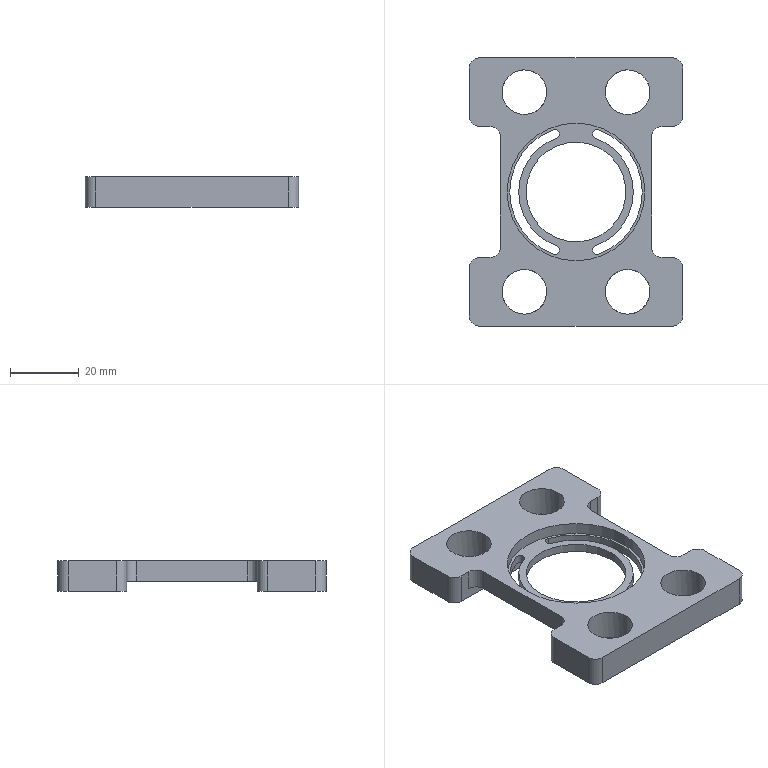NC program | NX | posted with a generic post | part box 62 x 78 x 9 mm
Lines 793 to 1620 of 3044:
(ZLEVEL_PROFILE_COPY_1 , TOOL : D2)
N1548 T02 M6
N1550 G54
N1552 G17 G0 G90 X12.199 Y12.797 S9500 M3
N1554 G43 Z30. H2
N1556 Z-2.
N1558 G94 G1 X13.603 Y11.294 Z-2.108 F1000.
N1560 X15.071 Y9.243 Z-2.24
N1562 X16.233 Y7.004 Z-2.372
N1564 X16.621 Y5.939 Z-2.432
N1566 X16.709 Y5.884 Z-2.437
N1568 X16.854 Y5.84 Z-2.445
N1570 X16.991 Y5.833 Z-2.452
N1572 X17.196 Y6.113 Z-2.47
N1574 X16.791 Y7.226 Z-2.532
N1576 X15.852 Y9.103 Z-2.642
N1578 X14.704 Y10.86 Z-2.752
N1580 X14.035 Y11.665 Z-2.807
N1582 X13.998 Y11.71 Z-2.81
N1584 X13.326 Y12.513 Z-2.865
N1586 X11.169 Y14.471 Z-3.018
N1588 X8.728 Y16.062 Z-3.171
N1590 X6.066 Y17.244 Z-3.323
N1592 X5.014 Y17.548 Z-3.381
N1594 X4.008 Y17.835 Z-3.435
N1596 X1.954 Y18.175 Z-3.545
N1598 X0.908 Y18.227 Z-3.599
N1600 X0.857 Y18.23 Z-3.602
N1602 X0.429 Y18.25 Z-3.625
N1604 X0. Z-3.647
N1606 G3 X-0.857 Y18.23 R18.25 F2500.
N1608 G1 X-0.908 Y18.227
N1610 G3 X-13.998 Y11.71 R18.25
N1612 G1 X-14.035 Y11.665
N1614 G3 X-17.149 Y6.242 R18.25
N1616 X-16.97 Y5.857 R0.3
N1618 X-16.586 Y6.037 R0.3
N1620 G2 X16.586 Y6.037 R17.65
N1622 G1 X16.611 Y5.931
N1624 X16.709 Y5.884
N1626 X16.854 Y5.84
N1628 G3 X17.149 Y6.242 R0.3
N1630 X14.035 Y11.665 R18.25
N1632 G1 X13.998 Y11.71
N1634 G3 X0.908 Y18.227 R18.25
N1636 G1 X0.857 Y18.23
N1638 G3 X0. Y18.25 R18.25
N1640 G1 X-0.168 Y18.24 Z-3.65
N1642 X-0.337 Y18.232 Z-3.653
N1644 X-0.505 Y18.221 Z-3.656
N1646 X-0.673 Y18.213 Z-3.659
N1648 X-0.841 Y18.203 Z-3.662
N1650 X-1.009 Y18.195 Z-3.665
N1652 X-1.177 Y18.184 Z-3.668
N1654 X-1.345 Y18.176 Z-3.671
N1656 X-1.513 Y18.166 Z-3.674
N1658 X-1.681 Y18.157 Z-3.676
N1660 X-1.849 Y18.147 Z-3.679
N1662 X-2.018 Y18.138 Z-3.682
N1664 X-2.184 Y18.111 Z-3.685
N1666 X-2.35 Y18.083 Z-3.688
N1668 X-2.516 Y18.054 Z-3.691
N1670 X-2.683 Y18.027 Z-3.694
N1672 X-2.848 Y17.998 Z-3.697
N1674 X-3.015 Y17.971 Z-3.7
N1676 X-3.18 Y17.943 Z-3.703
N1678 X-3.346 Y17.915 Z-3.706
N1680 X-3.512 Y17.887 Z-3.709
N1682 X-3.678 Y17.86 Z-3.712
N1684 X-3.845 Y17.831 Z-3.715
N1686 X-4.011 Y17.804 Z-3.718
N1688 X-4.173 Y17.758 Z-3.721
N1690 X-4.335 Y17.712 Z-3.724
N1692 X-4.497 Y17.665 Z-3.726
N1694 X-4.659 Y17.62 Z-3.729
N1696 X-4.821 Y17.573 Z-3.732
N1698 X-4.983 Y17.528 Z-3.735
N1700 X-5.145 Y17.481 Z-3.738
N1702 X-5.307 Y17.436 Z-3.741
N1704 X-5.469 Y17.39 Z-3.744
N1706 X-5.63 Y17.342 Z-3.747
N1708 X-5.793 Y17.297 Z-3.75
N1710 X-5.955 Y17.251 Z-3.753
N1712 X-6.111 Y17.188 Z-3.756
N1714 X-6.267 Y17.124 Z-3.759
N1716 X-6.423 Y17.061 Z-3.762
N1718 X-6.579 Y16.997 Z-3.765
N1720 X-6.734 Y16.932 Z-3.768
N1722 X-6.891 Y16.87 Z-3.771
N1724 X-7.046 Y16.805 Z-3.774
N1726 X-7.202 Y16.742 Z-3.776
N1728 X-7.357 Y16.677 Z-3.779
N1730 X-7.513 Y16.614 Z-3.782
N1732 X-7.669 Y16.549 Z-3.785
N1734 X-7.826 Y16.487 Z-3.788
N1736 X-7.975 Y16.408 Z-3.791
N1738 X-8.129 Y16.34 Z-3.794
N1740 G3 X-13.998 Y11.71 R18.25
N1742 G1 X-14.035 Y11.665
N1744 G3 X-17.149 Y6.242 R18.25
N1746 X-16.97 Y5.857 R0.3
N1748 X-16.586 Y6.037 R0.3
N1750 G2 X16.586 Y6.037 R17.65
N1752 G1 X16.611 Y5.931
N1754 X16.709 Y5.884
N1756 X16.854 Y5.84
N1758 G3 X17.149 Y6.242 R0.3
N1760 X14.035 Y11.665 R18.25
N1762 G1 X13.998 Y11.71
N1764 G3 X0.908 Y18.227 R18.25
N1766 G1 X0.857 Y18.23
N1768 G3 X0. Y18.25 R18.25
N1770 G1 X-0.168 Y18.24 Z-3.797
N1772 X-0.337 Y18.232 Z-3.8
N1774 X-0.505 Y18.221 Z-3.803
N1776 X-0.673 Y18.213 Z-3.806
N1778 X-0.841 Y18.203 Z-3.809
N1780 X-1.009 Y18.195 Z-3.812
N1782 X-1.177 Y18.184 Z-3.815
N1784 X-1.345 Y18.176 Z-3.818
N1786 X-1.513 Y18.165 Z-3.821
N1788 X-1.681 Y18.157 Z-3.824
N1790 X-1.849 Y18.147 Z-3.826
N1792 X-2.018 Y18.138 Z-3.829
N1794 X-2.184 Y18.111 Z-3.832
N1796 X-2.35 Y18.083 Z-3.835
N1798 X-2.516 Y18.054 Z-3.838
N1800 X-2.683 Y18.027 Z-3.841
N1802 X-2.848 Y17.998 Z-3.844
N1804 X-3.015 Y17.971 Z-3.847
N1806 X-3.18 Y17.943 Z-3.85
N1808 X-3.346 Y17.915 Z-3.853
N1810 X-3.512 Y17.887 Z-3.856
N1812 X-3.678 Y17.86 Z-3.859
N1814 X-3.845 Y17.831 Z-3.862
N1816 X-4.011 Y17.804 Z-3.865
N1818 X-4.173 Y17.758 Z-3.868
N1820 X-4.335 Y17.712 Z-3.871
N1822 X-4.497 Y17.665 Z-3.874
N1824 X-4.659 Y17.62 Z-3.876
N1826 X-4.821 Y17.573 Z-3.879
N1828 X-4.983 Y17.528 Z-3.882
N1830 X-5.145 Y17.481 Z-3.885
N1832 X-5.307 Y17.436 Z-3.888
N1834 X-5.469 Y17.39 Z-3.891
N1836 X-5.63 Y17.342 Z-3.894
N1838 X-5.793 Y17.297 Z-3.897
N1840 X-5.955 Y17.251 Z-3.9
N1842 X-6.111 Y17.188 Z-3.903
N1844 X-6.267 Y17.124 Z-3.906
N1846 X-6.423 Y17.061 Z-3.909
N1848 X-6.579 Y16.997 Z-3.912
N1850 X-6.734 Y16.932 Z-3.915
N1852 X-6.891 Y16.869 Z-3.918
N1854 X-7.046 Y16.805 Z-3.921
N1856 X-7.202 Y16.742 Z-3.924
N1858 X-7.357 Y16.677 Z-3.926
N1860 X-7.513 Y16.614 Z-3.929
N1862 X-7.669 Y16.549 Z-3.932
N1864 X-7.826 Y16.487 Z-3.935
N1866 X-7.975 Y16.408 Z-3.938
N1868 X-8.129 Y16.34 Z-3.941
N1870 G3 X-13.998 Y11.71 R18.25
N1872 G1 X-14.035 Y11.665
N1874 G3 X-17.149 Y6.242 R18.25
N1876 X-16.97 Y5.857 R0.3
N1878 X-16.586 Y6.037 R0.3
N1880 G2 X16.586 Y6.037 R17.65
N1882 G1 X16.611 Y5.931
N1884 X16.709 Y5.884
N1886 X16.854 Y5.84
N1888 G3 X17.149 Y6.242 R0.3
N1890 X14.035 Y11.665 R18.25
N1892 G1 X13.998 Y11.71
N1894 G3 X0.908 Y18.227 R18.25
N1896 G1 X0.857 Y18.23
N1898 G3 X0. Y18.25 R18.25
N1900 G1 X-0.168 Y18.24 Z-3.944
N1902 X-0.337 Y18.232 Z-3.947
N1904 X-0.505 Y18.221 Z-3.95
N1906 X-0.673 Y18.213 Z-3.953
N1908 X-0.841 Y18.203 Z-3.956
N1910 X-1.009 Y18.195 Z-3.959
N1912 X-1.177 Y18.184 Z-3.962
N1914 X-1.345 Y18.176 Z-3.965
N1916 X-1.513 Y18.165 Z-3.968
N1918 X-1.681 Y18.157 Z-3.971
N1920 X-1.849 Y18.147 Z-3.974
N1922 X-2.018 Y18.138 Z-3.976
N1924 X-2.184 Y18.111 Z-3.979
N1926 X-2.35 Y18.083 Z-3.982
N1928 X-2.516 Y18.054 Z-3.985
N1930 X-2.683 Y18.027 Z-3.988
N1932 X-2.848 Y17.998 Z-3.991
N1934 X-3.015 Y17.971 Z-3.994
N1936 X-3.18 Y17.943 Z-3.997
N1938 X-3.346 Y17.915 Z-4.
N1940 X-3.512 Y17.887 Z-4.003
N1942 X-3.678 Y17.86 Z-4.006
N1944 X-3.845 Y17.831 Z-4.009
N1946 X-4.011 Y17.803 Z-4.012
N1948 X-4.173 Y17.758 Z-4.015
N1950 X-4.335 Y17.712 Z-4.018
N1952 X-4.497 Y17.665 Z-4.021
N1954 X-4.659 Y17.62 Z-4.024
N1956 X-4.821 Y17.573 Z-4.026
N1958 X-4.983 Y17.528 Z-4.029
N1960 X-5.145 Y17.481 Z-4.032
N1962 X-5.307 Y17.436 Z-4.035
N1964 X-5.469 Y17.39 Z-4.038
N1966 X-5.63 Y17.342 Z-4.041
N1968 X-5.793 Y17.297 Z-4.044
N1970 X-5.955 Y17.251 Z-4.047
N1972 X-6.111 Y17.188 Z-4.05
N1974 X-6.267 Y17.124 Z-4.053
N1976 X-6.423 Y17.061 Z-4.056
N1978 X-6.579 Y16.997 Z-4.059
N1980 X-6.734 Y16.932 Z-4.062
N1982 X-6.891 Y16.869 Z-4.065
N1984 X-7.046 Y16.805 Z-4.068
N1986 X-7.202 Y16.742 Z-4.071
N1988 X-7.357 Y16.677 Z-4.074
N1990 X-7.513 Y16.614 Z-4.076
N1992 X-7.669 Y16.549 Z-4.079
N1994 X-7.826 Y16.486 Z-4.082
N1996 X-7.975 Y16.408 Z-4.085
N1998 X-8.129 Y16.34 Z-4.088
N2000 G3 X-13.998 Y11.71 R18.25
N2002 G1 X-14.035 Y11.665
N2004 G3 X-17.149 Y6.242 R18.25
N2006 X-16.97 Y5.857 R0.3
N2008 X-16.586 Y6.037 R0.3
N2010 G2 X16.586 Y6.037 R17.65
N2012 G1 X16.611 Y5.931
N2014 X16.709 Y5.884
N2016 X16.854 Y5.84
N2018 G3 X17.149 Y6.242 R0.3
N2020 X14.035 Y11.665 R18.25
N2022 G1 X13.998 Y11.71
N2024 G3 X0.908 Y18.227 R18.25
N2026 G1 X0.857 Y18.23
N2028 G3 X0. Y18.25 R18.25
N2030 G1 X-0.168 Y18.24 Z-4.091
N2032 X-0.337 Y18.232 Z-4.094
N2034 X-0.505 Y18.221 Z-4.097
N2036 X-0.673 Y18.213 Z-4.1
N2038 X-0.841 Y18.203 Z-4.103
N2040 X-1.009 Y18.194 Z-4.106
N2042 X-1.177 Y18.184 Z-4.109
N2044 X-1.345 Y18.176 Z-4.112
N2046 X-1.513 Y18.165 Z-4.115
N2048 X-1.681 Y18.157 Z-4.118
N2050 X-1.849 Y18.147 Z-4.121
N2052 X-2.018 Y18.138 Z-4.124
N2054 X-2.184 Y18.111 Z-4.126
N2056 X-2.35 Y18.083 Z-4.129
N2058 X-2.516 Y18.054 Z-4.132
N2060 X-2.683 Y18.027 Z-4.135
N2062 X-2.848 Y17.998 Z-4.138
N2064 X-3.014 Y17.971 Z-4.141
N2066 X-3.18 Y17.943 Z-4.144
N2068 X-3.346 Y17.915 Z-4.147
N2070 X-3.512 Y17.887 Z-4.15
N2072 X-3.678 Y17.86 Z-4.153
N2074 X-3.845 Y17.831 Z-4.156
N2076 X-4.011 Y17.803 Z-4.159
N2078 X-4.173 Y17.758 Z-4.162
N2080 X-4.335 Y17.712 Z-4.165
N2082 X-4.497 Y17.665 Z-4.168
N2084 X-4.659 Y17.62 Z-4.171
N2086 X-4.821 Y17.573 Z-4.174
N2088 X-4.983 Y17.528 Z-4.176
N2090 X-5.145 Y17.481 Z-4.179
N2092 X-5.307 Y17.436 Z-4.182
N2094 X-5.469 Y17.389 Z-4.185
N2096 X-5.63 Y17.342 Z-4.188
N2098 X-5.793 Y17.297 Z-4.191
N2100 X-5.955 Y17.251 Z-4.194
N2102 X-6.111 Y17.188 Z-4.197
N2104 X-6.267 Y17.124 Z-4.2
N2106 X-6.423 Y17.061 Z-4.203
N2108 X-6.579 Y16.997 Z-4.206
N2110 X-6.734 Y16.932 Z-4.209
N2112 X-6.891 Y16.869 Z-4.212
N2114 X-7.046 Y16.805 Z-4.215
N2116 X-7.202 Y16.742 Z-4.218
N2118 X-7.357 Y16.677 Z-4.221
N2120 X-7.513 Y16.614 Z-4.224
N2122 X-7.669 Y16.549 Z-4.226
N2124 X-7.826 Y16.486 Z-4.229
N2126 X-7.975 Y16.408 Z-4.232
N2128 X-8.129 Y16.34 Z-4.235
N2130 G3 X-13.998 Y11.71 R18.25
N2132 G1 X-14.035 Y11.665
N2134 G3 X-17.149 Y6.242 R18.25
N2136 X-16.97 Y5.857 R0.3
N2138 X-16.586 Y6.037 R0.3
N2140 G2 X16.586 Y6.037 R17.65
N2142 G1 X16.611 Y5.931
N2144 X16.709 Y5.884
N2146 X16.854 Y5.84
N2148 G3 X17.149 Y6.242 R0.3
N2150 X14.035 Y11.665 R18.25
N2152 G1 X13.998 Y11.71
N2154 G3 X0.908 Y18.227 R18.25
N2156 G1 X0.857 Y18.23
N2158 G3 X0. Y18.25 R18.25
N2160 G1 X-0.168 Y18.24 Z-4.238
N2162 X-0.337 Y18.232 Z-4.241
N2164 X-0.505 Y18.221 Z-4.244
N2166 X-0.673 Y18.213 Z-4.247
N2168 X-0.841 Y18.203 Z-4.25
N2170 X-1.009 Y18.194 Z-4.253
N2172 X-1.177 Y18.184 Z-4.256
N2174 X-1.345 Y18.176 Z-4.259
N2176 X-1.513 Y18.165 Z-4.262
N2178 X-1.681 Y18.157 Z-4.265
N2180 X-1.849 Y18.147 Z-4.268
N2182 X-2.018 Y18.138 Z-4.271
N2184 X-2.184 Y18.111 Z-4.274
N2186 X-2.35 Y18.083 Z-4.276
N2188 X-2.516 Y18.054 Z-4.279
N2190 X-2.683 Y18.027 Z-4.282
N2192 X-2.848 Y17.998 Z-4.285
N2194 X-3.014 Y17.971 Z-4.288
N2196 X-3.18 Y17.943 Z-4.291
N2198 X-3.346 Y17.915 Z-4.294
N2200 X-3.512 Y17.887 Z-4.297
N2202 X-3.678 Y17.86 Z-4.3
N2204 X-3.844 Y17.831 Z-4.303
N2206 X-4.011 Y17.803 Z-4.306
N2208 X-4.173 Y17.758 Z-4.309
N2210 X-4.335 Y17.712 Z-4.312
N2212 X-4.497 Y17.665 Z-4.315
N2214 X-4.659 Y17.62 Z-4.318
N2216 X-4.821 Y17.573 Z-4.321
N2218 X-4.983 Y17.528 Z-4.324
N2220 X-5.145 Y17.481 Z-4.326
N2222 X-5.307 Y17.435 Z-4.329
N2224 X-5.469 Y17.389 Z-4.332
N2226 X-5.63 Y17.342 Z-4.335
N2228 X-5.793 Y17.297 Z-4.338
N2230 X-5.955 Y17.251 Z-4.341
N2232 X-6.111 Y17.188 Z-4.344
N2234 X-6.267 Y17.124 Z-4.347
N2236 X-6.423 Y17.061 Z-4.35
N2238 X-6.579 Y16.997 Z-4.353
N2240 X-6.734 Y16.932 Z-4.356
N2242 X-6.891 Y16.869 Z-4.359
N2244 X-7.046 Y16.805 Z-4.362
N2246 X-7.202 Y16.742 Z-4.365
N2248 X-7.357 Y16.677 Z-4.368
N2250 X-7.513 Y16.614 Z-4.371
N2252 X-7.669 Y16.549 Z-4.374
N2254 X-7.826 Y16.486 Z-4.376
N2256 X-7.975 Y16.408 Z-4.379
N2258 X-8.129 Y16.34 Z-4.382
N2260 G3 X-13.998 Y11.71 R18.25
N2262 G1 X-14.035 Y11.665
N2264 G3 X-17.149 Y6.242 R18.25
N2266 X-16.97 Y5.857 R0.3
N2268 X-16.586 Y6.037 R0.3
N2270 G2 X16.586 Y6.037 R17.65
N2272 G1 X16.611 Y5.931
N2274 X16.709 Y5.884
N2276 X16.854 Y5.84
N2278 G3 X17.149 Y6.242 R0.3
N2280 X14.035 Y11.665 R18.25
N2282 G1 X13.998 Y11.71
N2284 G3 X0.908 Y18.227 R18.25
N2286 G1 X0.857 Y18.23
N2288 G3 X0. Y18.25 R18.25
N2290 G1 X-0.168 Y18.24 Z-4.385
N2292 X-0.337 Y18.232 Z-4.388
N2294 X-0.505 Y18.221 Z-4.391
N2296 X-0.673 Y18.213 Z-4.394
N2298 X-0.841 Y18.203 Z-4.397
N2300 X-1.009 Y18.194 Z-4.4
N2302 X-1.177 Y18.184 Z-4.403
N2304 X-1.345 Y18.176 Z-4.406
N2306 X-1.513 Y18.165 Z-4.409
N2308 X-1.681 Y18.157 Z-4.412
N2310 X-1.849 Y18.147 Z-4.415
N2312 X-2.018 Y18.138 Z-4.418
N2314 X-2.184 Y18.111 Z-4.421
N2316 X-2.35 Y18.083 Z-4.424
N2318 X-2.516 Y18.054 Z-4.426
N2320 X-2.683 Y18.027 Z-4.429
N2322 X-2.848 Y17.998 Z-4.432
N2324 X-3.014 Y17.971 Z-4.435
N2326 X-3.18 Y17.942 Z-4.438
N2328 X-3.346 Y17.915 Z-4.441
N2330 X-3.512 Y17.887 Z-4.444
N2332 X-3.678 Y17.86 Z-4.447
N2334 X-3.844 Y17.831 Z-4.45
N2336 X-4.011 Y17.803 Z-4.453
N2338 X-4.173 Y17.758 Z-4.456
N2340 X-4.335 Y17.712 Z-4.459
N2342 X-4.497 Y17.665 Z-4.462
N2344 X-4.659 Y17.62 Z-4.465
N2346 X-4.821 Y17.573 Z-4.468
N2348 X-4.983 Y17.528 Z-4.471
N2350 X-5.145 Y17.481 Z-4.474
N2352 X-5.307 Y17.435 Z-4.476
N2354 X-5.469 Y17.389 Z-4.479
N2356 X-5.63 Y17.342 Z-4.482
N2358 X-5.793 Y17.297 Z-4.485
N2360 X-5.955 Y17.251 Z-4.488
N2362 X-6.111 Y17.188 Z-4.491
N2364 X-6.267 Y17.124 Z-4.494
N2366 X-6.423 Y17.061 Z-4.497
N2368 X-6.579 Y16.997 Z-4.5
N2370 X-6.734 Y16.932 Z-4.503
N2372 X-6.891 Y16.869 Z-4.506
N2374 X-7.046 Y16.805 Z-4.509
N2376 X-7.202 Y16.742 Z-4.512
N2378 X-7.357 Y16.677 Z-4.515
N2380 X-7.513 Y16.614 Z-4.518
N2382 X-7.669 Y16.549 Z-4.521
N2384 X-7.826 Y16.486 Z-4.524
N2386 X-7.975 Y16.407 Z-4.526
N2388 X-8.129 Y16.34 Z-4.529
N2390 G3 X-13.998 Y11.71 R18.25
N2392 G1 X-14.035 Y11.665
N2394 G3 X-17.149 Y6.242 R18.25
N2396 X-16.97 Y5.857 R0.3
N2398 X-16.586 Y6.037 R0.3
N2400 G2 X16.586 Y6.037 R17.65
N2402 G1 X16.611 Y5.931
N2404 X16.709 Y5.884
N2406 X16.854 Y5.84
N2408 G3 X17.149 Y6.242 R0.3
N2410 X14.035 Y11.665 R18.25
N2412 G1 X13.998 Y11.71
N2414 G3 X0.908 Y18.227 R18.25
N2416 G1 X0.857 Y18.23
N2418 G3 X0. Y18.25 R18.25
N2420 G1 X-0.168 Y18.24 Z-4.532
N2422 X-0.337 Y18.232 Z-4.535
N2424 X-0.505 Y18.221 Z-4.538
N2426 X-0.673 Y18.213 Z-4.541
N2428 X-0.841 Y18.203 Z-4.544
N2430 X-1.009 Y18.194 Z-4.547
N2432 X-1.177 Y18.184 Z-4.55
N2434 X-1.345 Y18.176 Z-4.553
N2436 X-1.513 Y18.165 Z-4.556
N2438 X-1.681 Y18.157 Z-4.559
N2440 X-1.849 Y18.147 Z-4.562
N2442 X-2.018 Y18.138 Z-4.565
N2444 X-2.184 Y18.111 Z-4.568
N2446 X-2.35 Y18.083 Z-4.571
N2448 X-2.516 Y18.054 Z-4.574
N2450 X-2.683 Y18.027 Z-4.576
N2452 X-2.848 Y17.998 Z-4.579
N2454 X-3.014 Y17.971 Z-4.582
N2456 X-3.18 Y17.942 Z-4.585
N2458 X-3.346 Y17.915 Z-4.588
N2460 X-3.512 Y17.887 Z-4.591
N2462 X-3.678 Y17.86 Z-4.594
N2464 X-3.844 Y17.831 Z-4.597
N2466 X-4.011 Y17.803 Z-4.6
N2468 X-4.173 Y17.758 Z-4.603
N2470 X-4.335 Y17.712 Z-4.606
N2472 X-4.497 Y17.666 Z-4.609
N2474 X-4.659 Y17.62 Z-4.612
N2476 X-4.821 Y17.573 Z-4.615
N2478 X-4.983 Y17.528 Z-4.618
N2480 X-5.145 Y17.481 Z-4.621
N2482 X-5.307 Y17.435 Z-4.624
N2484 X-5.469 Y17.389 Z-4.626
N2486 X-5.63 Y17.342 Z-4.629
N2488 X-5.793 Y17.297 Z-4.632
N2490 X-5.955 Y17.251 Z-4.635
N2492 X-6.111 Y17.188 Z-4.638
N2494 X-6.267 Y17.124 Z-4.641
N2496 X-6.423 Y17.061 Z-4.644
N2498 X-6.579 Y16.997 Z-4.647
N2500 X-6.734 Y16.932 Z-4.65
N2502 X-6.891 Y16.869 Z-4.653
N2504 X-7.046 Y16.805 Z-4.656
N2506 X-7.202 Y16.742 Z-4.659
N2508 X-7.357 Y16.677 Z-4.662
N2510 X-7.513 Y16.614 Z-4.665
N2512 X-7.669 Y16.549 Z-4.668
N2514 X-7.826 Y16.486 Z-4.671
N2516 X-7.975 Y16.407 Z-4.674
N2518 X-8.129 Y16.34 Z-4.676
N2520 G3 X-13.998 Y11.71 R18.25
N2522 G1 X-14.035 Y11.665
N2524 G3 X-17.149 Y6.242 R18.25
N2526 X-16.97 Y5.857 R0.3
N2528 X-16.586 Y6.037 R0.3
N2530 G2 X16.586 Y6.037 R17.65
N2532 G1 X16.611 Y5.931
N2534 X16.709 Y5.884
N2536 X16.854 Y5.84
N2538 G3 X17.149 Y6.242 R0.3
N2540 X14.035 Y11.665 R18.25
N2542 G1 X13.998 Y11.71
N2544 G3 X0.908 Y18.227 R18.25
N2546 G1 X0.857 Y18.23
N2548 G3 X0. Y18.25 R18.25
N2550 G1 X-0.168 Y18.24 Z-4.679
N2552 X-0.337 Y18.232 Z-4.682
N2554 X-0.505 Y18.221 Z-4.685
N2556 X-0.673 Y18.213 Z-4.688
N2558 X-0.841 Y18.203 Z-4.691
N2560 X-1.009 Y18.194 Z-4.694
N2562 X-1.177 Y18.184 Z-4.697
N2564 X-1.345 Y18.176 Z-4.7
N2566 X-1.513 Y18.165 Z-4.703
N2568 X-1.681 Y18.157 Z-4.706
N2570 X-1.849 Y18.147 Z-4.709
N2572 X-2.018 Y18.138 Z-4.712
N2574 X-2.184 Y18.111 Z-4.715
N2576 X-2.35 Y18.083 Z-4.718
N2578 X-2.516 Y18.054 Z-4.721
N2580 X-2.683 Y18.027 Z-4.724
N2582 X-2.848 Y17.998 Z-4.726
N2584 X-3.014 Y17.971 Z-4.729
N2586 X-3.18 Y17.942 Z-4.732
N2588 X-3.346 Y17.915 Z-4.735
N2590 X-3.512 Y17.887 Z-4.738
N2592 X-3.678 Y17.86 Z-4.741
N2594 X-3.844 Y17.831 Z-4.744
N2596 X-4.011 Y17.803 Z-4.747
N2598 X-4.173 Y17.758 Z-4.75
N2600 X-4.335 Y17.712 Z-4.753
N2602 X-4.497 Y17.666 Z-4.756
N2604 X-4.659 Y17.62 Z-4.759
N2606 X-4.821 Y17.573 Z-4.762
N2608 X-4.983 Y17.528 Z-4.765
N2610 X-5.145 Y17.481 Z-4.768
N2612 X-5.307 Y17.435 Z-4.771
N2614 X-5.469 Y17.389 Z-4.774
N2616 X-5.63 Y17.342 Z-4.776
N2618 X-5.793 Y17.297 Z-4.779
N2620 X-5.955 Y17.251 Z-4.782
N2622 X-6.111 Y17.188 Z-4.785
N2624 X-6.267 Y17.124 Z-4.788
N2626 X-6.423 Y17.061 Z-4.791
N2628 X-6.579 Y16.997 Z-4.794
N2630 X-6.734 Y16.932 Z-4.797
N2632 X-6.89 Y16.869 Z-4.8
N2634 X-7.046 Y16.805 Z-4.803
N2636 X-7.202 Y16.742 Z-4.806
N2638 X-7.358 Y16.678 Z-4.809
N2640 X-7.513 Y16.614 Z-4.812
N2642 X-7.669 Y16.549 Z-4.815
N2644 X-7.826 Y16.486 Z-4.818
N2646 X-7.975 Y16.407 Z-4.821
N2648 X-8.129 Y16.34 Z-4.824
N2650 G3 X-13.998 Y11.71 R18.25
N2652 G1 X-14.035 Y11.665
N2654 G3 X-17.149 Y6.242 R18.25
N2656 X-16.97 Y5.857 R0.3
N2658 X-16.586 Y6.037 R0.3
N2660 G2 X16.586 Y6.037 R17.65
N2662 G1 X16.611 Y5.931
N2664 X16.709 Y5.884
N2666 X16.854 Y5.84
N2668 G3 X17.149 Y6.242 R0.3
N2670 X14.035 Y11.665 R18.25
N2672 G1 X13.998 Y11.71
N2674 G3 X0.908 Y18.227 R18.25
N2676 G1 X0.857 Y18.23
N2678 G3 X0. Y18.25 R18.25
N2680 G1 X-0.168 Y18.24 Z-4.826
N2682 X-0.337 Y18.232 Z-4.829
N2684 X-0.505 Y18.221 Z-4.832
N2686 X-0.673 Y18.213 Z-4.835
N2688 X-0.841 Y18.203 Z-4.838
N2690 X-1.009 Y18.194 Z-4.841
N2692 X-1.177 Y18.184 Z-4.844
N2694 X-1.345 Y18.176 Z-4.847
N2696 X-1.513 Y18.165 Z-4.85
N2698 X-1.681 Y18.157 Z-4.853
N2700 X-1.849 Y18.146 Z-4.856
N2702 X-2.018 Y18.138 Z-4.859
N2704 X-2.184 Y18.111 Z-4.862
N2706 X-2.35 Y18.083 Z-4.865
N2708 X-2.516 Y18.054 Z-4.868
N2710 X-2.683 Y18.027 Z-4.871
N2712 X-2.848 Y17.998 Z-4.874
N2714 X-3.014 Y17.971 Z-4.876
N2716 X-3.18 Y17.942 Z-4.879
N2718 X-3.346 Y17.915 Z-4.882
N2720 X-3.512 Y17.887 Z-4.885
N2722 X-3.678 Y17.86 Z-4.888
N2724 X-3.844 Y17.831 Z-4.891
N2726 X-4.011 Y17.803 Z-4.894
N2728 X-4.173 Y17.758 Z-4.897
N2730 X-4.335 Y17.712 Z-4.9
N2732 X-4.497 Y17.666 Z-4.903
N2734 X-4.659 Y17.62 Z-4.906
N2736 X-4.821 Y17.573 Z-4.909
N2738 X-4.983 Y17.528 Z-4.912
N2740 X-5.145 Y17.481 Z-4.915
N2742 X-5.307 Y17.435 Z-4.918
N2744 X-5.469 Y17.389 Z-4.921
N2746 X-5.63 Y17.342 Z-4.924
N2748 X-5.793 Y17.297 Z-4.926
N2750 X-5.955 Y17.251 Z-4.929
N2752 X-6.111 Y17.188 Z-4.932
N2754 X-6.267 Y17.124 Z-4.935
N2756 X-6.423 Y17.061 Z-4.938
N2758 X-6.579 Y16.997 Z-4.941
N2760 X-6.734 Y16.932 Z-4.944
N2762 X-6.89 Y16.869 Z-4.947
N2764 X-7.046 Y16.805 Z-4.95
N2766 X-7.202 Y16.742 Z-4.953
N2768 X-7.358 Y16.678 Z-4.956
N2770 X-7.513 Y16.614 Z-4.959
N2772 X-7.669 Y16.549 Z-4.962
N2774 X-7.826 Y16.486 Z-4.965
N2776 X-7.975 Y16.407 Z-4.968
N2778 X-8.129 Y16.34 Z-4.971
N2780 G3 X-13.998 Y11.71 R18.25
N2782 G1 X-14.035 Y11.665
N2784 G3 X-17.149 Y6.242 R18.25
N2786 X-16.97 Y5.857 R0.3
N2788 X-16.586 Y6.037 R0.3
N2790 G2 X16.586 Y6.037 R17.65
N2792 G1 X16.611 Y5.931
N2794 X16.709 Y5.884
N2796 X16.854 Y5.84
N2798 G3 X17.149 Y6.242 R0.3
N2800 X14.035 Y11.665 R18.25
N2802 G1 X13.998 Y11.71
N2804 G3 X0.908 Y18.227 R18.25
N2806 G1 X0.857 Y18.23
N2808 G3 X0. Y18.25 R18.25
N2810 G1 X-0.168 Y18.24 Z-4.974
N2812 X-0.337 Y18.232 Z-4.976
N2814 X-0.505 Y18.221 Z-4.979
N2816 X-0.673 Y18.213 Z-4.982
N2818 X-0.841 Y18.203 Z-4.985
N2820 X-1.009 Y18.194 Z-4.988
N2822 X-1.177 Y18.184 Z-4.991
N2824 X-1.345 Y18.175 Z-4.994
N2826 X-1.513 Y18.165 Z-4.997
N2828 X-1.681 Y18.157 Z-5.
N2830 X-1.849 Y18.146 Z-5.003
N2832 X-2.018 Y18.138 Z-5.006
N2834 X-2.184 Y18.111 Z-5.009
N2836 X-2.35 Y18.083 Z-5.012
N2838 X-2.516 Y18.054 Z-5.015
N2840 X-2.683 Y18.027 Z-5.018
N2842 X-2.848 Y17.998 Z-5.021
N2844 X-3.014 Y17.971 Z-5.024
N2846 X-3.18 Y17.942 Z-5.026
N2848 X-3.346 Y17.915 Z-5.029
N2850 X-3.512 Y17.887 Z-5.032
N2852 X-3.678 Y17.86 Z-5.035
N2854 X-3.844 Y17.831 Z-5.038
N2856 X-4.011 Y17.803 Z-5.041
N2858 X-4.173 Y17.758 Z-5.044
N2860 X-4.335 Y17.712 Z-5.047
N2862 X-4.497 Y17.666 Z-5.05
N2864 X-4.659 Y17.62 Z-5.053
N2866 X-4.821 Y17.573 Z-5.056
N2868 X-4.983 Y17.528 Z-5.059
N2870 X-5.145 Y17.481 Z-5.062
N2872 X-5.307 Y17.435 Z-5.065
N2874 X-5.469 Y17.389 Z-5.068
N2876 X-5.63 Y17.342 Z-5.071
N2878 X-5.793 Y17.297 Z-5.074
N2880 X-5.955 Y17.251 Z-5.076
N2882 X-6.111 Y17.188 Z-5.079
N2884 X-6.267 Y17.124 Z-5.082
N2886 X-6.423 Y17.061 Z-5.085
N2888 X-6.579 Y16.997 Z-5.088
N2890 X-6.734 Y16.932 Z-5.091
N2892 X-6.89 Y16.869 Z-5.094
N2894 X-7.046 Y16.805 Z-5.097
N2896 X-7.202 Y16.742 Z-5.1
N2898 X-7.358 Y16.678 Z-5.103
N2900 X-7.513 Y16.614 Z-5.106
N2902 X-7.67 Y16.55 Z-5.109
N2904 X-7.826 Y16.486 Z-5.112
N2906 X-7.975 Y16.407 Z-5.115
N2908 X-8.129 Y16.34 Z-5.118
N2910 G3 X-13.998 Y11.71 R18.25
N2912 G1 X-14.035 Y11.665
N2914 G3 X-17.149 Y6.242 R18.25
N2916 X-16.97 Y5.857 R0.3
N2918 X-16.586 Y6.037 R0.3
N2920 G2 X16.586 Y6.037 R17.65
N2922 G1 X16.611 Y5.931
N2924 X16.709 Y5.884
N2926 X16.854 Y5.84
N2928 G3 X17.149 Y6.242 R0.3
N2930 X14.035 Y11.665 R18.25
N2932 G1 X13.998 Y11.71
N2934 G3 X0.908 Y18.227 R18.25
N2936 G1 X0.857 Y18.23
N2938 G3 X0. Y18.25 R18.25
N2940 G1 X-0.168 Y18.241 Z-5.121
N2942 X-0.337 Y18.232 Z-5.124
N2944 X-0.505 Y18.221 Z-5.126
N2946 X-0.673 Y18.213 Z-5.129
N2948 X-0.841 Y18.203 Z-5.132
N2950 X-1.009 Y18.194 Z-5.135
N2952 X-1.177 Y18.184 Z-5.138
N2954 X-1.345 Y18.175 Z-5.141
N2956 X-1.513 Y18.165 Z-5.144
N2958 X-1.681 Y18.157 Z-5.147
N2960 X-1.849 Y18.146 Z-5.15
N2962 X-2.018 Y18.138 Z-5.153
N2964 X-2.184 Y18.111 Z-5.156
N2966 X-2.35 Y18.083 Z-5.159
N2968 X-2.516 Y18.054 Z-5.162
N2970 X-2.683 Y18.027 Z-5.165
N2972 X-2.848 Y17.998 Z-5.168
N2974 X-3.014 Y17.971 Z-5.171
N2976 X-3.18 Y17.942 Z-5.174
N2978 X-3.346 Y17.915 Z-5.176
N2980 X-3.512 Y17.887 Z-5.179
N2982 X-3.678 Y17.86 Z-5.182
N2984 X-3.844 Y17.831 Z-5.185
N2986 X-4.011 Y17.803 Z-5.188
N2988 X-4.173 Y17.758 Z-5.191
N2990 X-4.335 Y17.712 Z-5.194
N2992 X-4.497 Y17.666 Z-5.197
N2994 X-4.659 Y17.62 Z-5.2
N2996 X-4.821 Y17.573 Z-5.203
N2998 X-4.983 Y17.528 Z-5.206
N3000 X-5.145 Y17.481 Z-5.209
N3002 X-5.307 Y17.435 Z-5.212
N3004 X-5.469 Y17.389 Z-5.215
N3006 X-5.63 Y17.342 Z-5.218
N3008 X-5.793 Y17.297 Z-5.221
N3010 X-5.955 Y17.251 Z-5.224
N3012 X-6.111 Y17.188 Z-5.226
N3014 X-6.267 Y17.124 Z-5.229
N3016 X-6.423 Y17.061 Z-5.232
N3018 X-6.579 Y16.997 Z-5.235
N3020 X-6.734 Y16.932 Z-5.238
N3022 X-6.89 Y16.869 Z-5.241
N3024 X-7.046 Y16.805 Z-5.244
N3026 X-7.202 Y16.742 Z-5.247
N3028 X-7.358 Y16.678 Z-5.25
N3030 X-7.513 Y16.614 Z-5.253
N3032 X-7.67 Y16.55 Z-5.256
N3034 X-7.826 Y16.486 Z-5.259
N3036 X-7.974 Y16.407 Z-5.262
N3038 X-8.129 Y16.34 Z-5.265
N3040 G3 X-13.998 Y11.71 R18.25
N3042 G1 X-14.035 Y11.665
N3044 G3 X-17.149 Y6.242 R18.25
N3046 X-16.97 Y5.857 R0.3
N3048 X-16.586 Y6.037 R0.3
N3050 G2 X16.586 Y6.037 R17.65
N3052 G1 X16.611 Y5.931
N3054 X16.709 Y5.884
N3056 X16.854 Y5.84
N3058 G3 X17.149 Y6.242 R0.3
N3060 X14.035 Y11.665 R18.25
N3062 G1 X13.998 Y11.71
N3064 G3 X0.908 Y18.227 R18.25
N3066 G1 X0.857 Y18.23
N3068 G3 X0. Y18.25 R18.25
N3070 G1 X-0.168 Y18.241 Z-5.268
N3072 X-0.337 Y18.232 Z-5.271
N3074 X-0.505 Y18.221 Z-5.274
N3076 X-0.673 Y18.213 Z-5.276
N3078 X-0.841 Y18.203 Z-5.279
N3080 X-1.009 Y18.194 Z-5.282
N3082 X-1.177 Y18.184 Z-5.285
N3084 X-1.345 Y18.175 Z-5.288
N3086 X-1.513 Y18.165 Z-5.291
N3088 X-1.681 Y18.157 Z-5.294
N3090 X-1.849 Y18.146 Z-5.297
N3092 X-2.018 Y18.138 Z-5.3
N3094 X-2.184 Y18.111 Z-5.303
N3096 X-2.35 Y18.083 Z-5.306
N3098 X-2.516 Y18.054 Z-5.309
N3100 X-2.683 Y18.027 Z-5.312
N3102 X-2.848 Y17.998 Z-5.315
N3104 X-3.014 Y17.971 Z-5.318
N3106 X-3.18 Y17.942 Z-5.321
N3108 X-3.346 Y17.915 Z-5.324
N3110 X-3.512 Y17.886 Z-5.326
N3112 X-3.678 Y17.86 Z-5.329
N3114 X-3.844 Y17.831 Z-5.332
N3116 X-4.011 Y17.803 Z-5.335
N3118 X-4.173 Y17.758 Z-5.338
N3120 X-4.335 Y17.712 Z-5.341
N3122 X-4.497 Y17.666 Z-5.344
N3124 X-4.659 Y17.62 Z-5.347
N3126 X-4.821 Y17.573 Z-5.35
N3128 X-4.983 Y17.528 Z-5.353
N3130 X-5.145 Y17.481 Z-5.356
N3132 X-5.307 Y17.435 Z-5.359
N3134 X-5.469 Y17.389 Z-5.362
N3136 X-5.63 Y17.342 Z-5.365
N3138 X-5.793 Y17.297 Z-5.368
N3140 X-5.955 Y17.251 Z-5.371
N3142 X-6.111 Y17.188 Z-5.374
N3144 X-6.267 Y17.124 Z-5.376
N3146 X-6.423 Y17.061 Z-5.379
N3148 X-6.579 Y16.997 Z-5.382
N3150 X-6.734 Y16.932 Z-5.385
N3152 X-6.89 Y16.869 Z-5.388
N3154 X-7.046 Y16.805 Z-5.391
N3156 X-7.202 Y16.742 Z-5.394
N3158 X-7.358 Y16.678 Z-5.397
N3160 X-7.513 Y16.614 Z-5.4
N3162 X-7.669 Y16.55 Z-5.403
N3164 X-7.826 Y16.486 Z-5.406
N3166 X-7.974 Y16.407 Z-5.409
N3168 X-8.129 Y16.34 Z-5.412
N3170 G3 X-13.998 Y11.71 R18.25
N3172 G1 X-14.035 Y11.665
N3174 G3 X-17.149 Y6.242 R18.25
N3176 X-16.97 Y5.857 R0.3
N3178 X-16.586 Y6.037 R0.3
N3180 G2 X16.586 Y6.037 R17.65
N3182 G1 X16.611 Y5.931
N3184 X16.709 Y5.884
N3186 X16.854 Y5.84
N3188 G3 X17.149 Y6.242 R0.3
N3190 X14.035 Y11.665 R18.25
N3192 G1 X13.998 Y11.71
N3194 G3 X0.908 Y18.227 R18.25
N3196 G1 X0.857 Y18.23